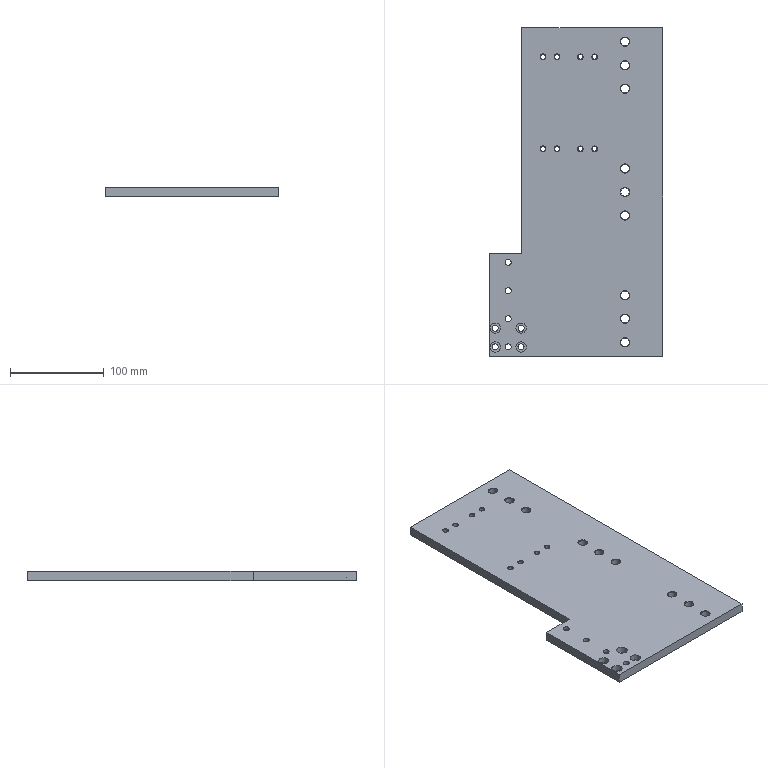Part | NX | features SIMPLE HOLE 25, SYMBOLIC_THREAD 17, DATUM_CSYS 10, HOLE PACKAGE 9, SKETCH 9, EXTRACT_FACE 6, CBORE_HOLE 4, Instance Feature 4, Pattern Feature 2, EXTRUDE 1 | 1 solid | 83 faces | box 184.5 x 350 x 10 mm | volume 549567 mm3 | cone 34 | cylinder 33 | plane 16 | commonest cylinder face diameters 9 x9 5.2 x8 6.5 x8 11 x8